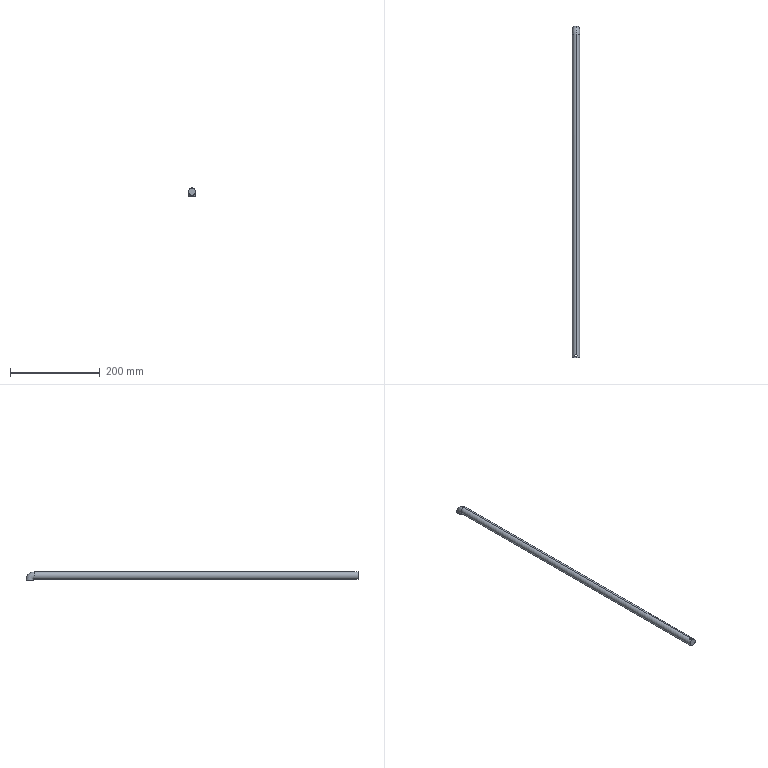Part | SolidWorks | features ICE 2, Sweep 1 | 1 solid | 19 faces | box 16 x 738 x 18 mm | volume 127006 mm3 | cylinder 12 | torus 4 | plane 3 | commonest cylinder face diameters 5 x4 6 x4 16 x4
STEP:
#1=CARTESIAN_POINT('',(-3.,0.,0.05));
#2=VERTEX_POINT('',#1);
#3=CARTESIAN_POINT('',(0.,3.,0.05));
#4=VERTEX_POINT('',#3);
#5=CARTESIAN_POINT('',(0.,0.,0.05));
#6=DIRECTION('',(0.,0.,-1.));
#7=DIRECTION('',(1.,0.,0.));
#8=AXIS2_PLACEMENT_3D('',#5,#6,#7);
#9=CIRCLE('',#8,3.);
#10=EDGE_CURVE('',#2,#4,#9,.T.);
#11=ORIENTED_EDGE('',*,*,#10,.T.);
#12=CARTESIAN_POINT('',(0.,-9.95,13.));
#13=VERTEX_POINT('',#12);
#14=CARTESIAN_POINT('',(0.,-9.95,0.05));
#15=DIRECTION('',(1.,0.,0.));
#16=DIRECTION('',(0.,0.,-1.));
#17=AXIS2_PLACEMENT_3D('',#14,#15,#16);
#18=CIRCLE('',#17,12.95);
#19=EDGE_CURVE('',#4,#13,#18,.T.);
#20=ORIENTED_EDGE('',*,*,#19,.T.);
#21=CARTESIAN_POINT('',(0.,-9.95,7.));
#22=VERTEX_POINT('',#21);
#23=CARTESIAN_POINT('',(0.,-9.95,10.));
#24=DIRECTION('',(0.,1.,0.));
#25=DIRECTION('',(1.,0.,0.));
#26=AXIS2_PLACEMENT_3D('',#23,#24,#25);
#27=CIRCLE('',#26,3.);
#28=EDGE_CURVE('',#22,#13,#27,.T.);
#29=ORIENTED_EDGE('',*,*,#28,.F.);
#30=CARTESIAN_POINT('',(0.,-3.,0.05));
#31=VERTEX_POINT('',#30);
#32=CARTESIAN_POINT('',(0.,-9.95,0.05));
#33=DIRECTION('',(1.,0.,0.));
#34=DIRECTION('',(0.,0.,-1.));
#35=AXIS2_PLACEMENT_3D('',#32,#33,#34);
#36=CIRCLE('',#35,6.95);
#37=EDGE_CURVE('',#31,#22,#36,.T.);
#38=ORIENTED_EDGE('',*,*,#37,.F.);
#39=CARTESIAN_POINT('',(0.,0.,0.05));
#40=DIRECTION('',(0.,0.,-1.));
#41=DIRECTION('',(1.,0.,0.));
#42=AXIS2_PLACEMENT_3D('',#39,#40,#41);
#43=CIRCLE('',#42,3.);
#44=EDGE_CURVE('',#31,#2,#43,.T.);
#45=ORIENTED_EDGE('',*,*,#44,.T.);
#46=EDGE_LOOP('',(#11,#20,#29,#38,#45));
#47=FACE_OUTER_BOUND('',#46,.T.);
#48=CARTESIAN_POINT('',(0.,-9.95,0.05));
#49=DIRECTION('',(1.,0.,0.));
#50=DIRECTION('',(0.,0.,-1.));
#51=AXIS2_PLACEMENT_3D('',#48,#49,#50);
#52=TOROIDAL_SURFACE('',#51,9.95,3.);
#53=ADVANCED_FACE('',(#47),#52,.F.);
#54=CARTESIAN_POINT('',(8.,0.,0.05));
#55=VERTEX_POINT('',#54);
#56=CARTESIAN_POINT('',(0.,8.,0.05));
#57=VERTEX_POINT('',#56);
#58=CARTESIAN_POINT('',(0.,0.,0.05));
#59=DIRECTION('',(0.,0.,1.));
#60=DIRECTION('',(1.,0.,0.));
#61=AXIS2_PLACEMENT_3D('',#58,#59,#60);
#62=CIRCLE('',#61,8.);
#63=EDGE_CURVE('',#55,#57,#62,.T.);
#64=ORIENTED_EDGE('',*,*,#63,.T.);
#65=CARTESIAN_POINT('',(0.,-9.95,18.));
#66=VERTEX_POINT('',#65);
#67=CARTESIAN_POINT('',(0.,-9.95,0.05));
#68=DIRECTION('',(1.,0.,0.));
#69=DIRECTION('',(0.,0.,-1.));
#70=AXIS2_PLACEMENT_3D('',#67,#68,#69);
#71=CIRCLE('',#70,17.95);
#72=EDGE_CURVE('',#57,#66,#71,.T.);
#73=ORIENTED_EDGE('',*,*,#72,.T.);
#74=CARTESIAN_POINT('',(0.,-9.95,2.));
#75=VERTEX_POINT('',#74);
#76=CARTESIAN_POINT('',(0.,-9.95,10.));
#77=DIRECTION('',(0.,-1.,0.));
#78=DIRECTION('',(1.,0.,0.));
#79=AXIS2_PLACEMENT_3D('',#76,#77,#78);
#80=CIRCLE('',#79,8.);
#81=EDGE_CURVE('',#75,#66,#80,.T.);
#82=ORIENTED_EDGE('',*,*,#81,.F.);
#83=CARTESIAN_POINT('',(0.,-8.,0.05));
#84=VERTEX_POINT('',#83);
#85=CARTESIAN_POINT('',(0.,-9.95,0.05));
#86=DIRECTION('',(1.,0.,0.));
#87=DIRECTION('',(0.,0.,-1.));
#88=AXIS2_PLACEMENT_3D('',#85,#86,#87);
#89=CIRCLE('',#88,1.95);
#90=EDGE_CURVE('',#84,#75,#89,.T.);
#91=ORIENTED_EDGE('',*,*,#90,.F.);
#92=CARTESIAN_POINT('',(0.,0.,0.05));
#93=DIRECTION('',(0.,0.,1.));
#94=DIRECTION('',(1.,0.,0.));
#95=AXIS2_PLACEMENT_3D('',#92,#93,#94);
#96=CIRCLE('',#95,8.);
#97=EDGE_CURVE('',#84,#55,#96,.T.);
#98=ORIENTED_EDGE('',*,*,#97,.T.);
#99=EDGE_LOOP('',(#64,#73,#82,#91,#98));
#100=FACE_OUTER_BOUND('',#99,.T.);
#101=CARTESIAN_POINT('',(0.,-9.95,0.05));
#102=DIRECTION('',(1.,0.,0.));
#103=DIRECTION('',(0.,0.,-1.));
#104=AXIS2_PLACEMENT_3D('',#101,#102,#103);
#105=TOROIDAL_SURFACE('',#104,9.95,8.);
#106=ADVANCED_FACE('',(#100),#105,.T.);
#107=CARTESIAN_POINT('',(0.,-727.,2.));
#108=VERTEX_POINT('',#107);
#109=CARTESIAN_POINT('',(-2.5,-724.5,2.401));
#110=VERTEX_POINT('',#109);
#111=CARTESIAN_POINT('',(0.,-727.,2.));
#112=CARTESIAN_POINT('',(-0.1638,-727.,2.));
#113=CARTESIAN_POINT('',(-0.3284,-726.984,2.005));
#114=CARTESIAN_POINT('',(-0.6528,-726.919,2.025));
#115=CARTESIAN_POINT('',(-0.8091,-726.871,2.04));
#116=CARTESIAN_POINT('',(-1.111,-726.746,2.076));
#117=CARTESIAN_POINT('',(-1.257,-726.667,2.098));
#118=CARTESIAN_POINT('',(-1.527,-726.486,2.146));
#119=CARTESIAN_POINT('',(-1.652,-726.383,2.172));
#120=CARTESIAN_POINT('',(-1.883,-726.152,2.224));
#121=CARTESIAN_POINT('',(-1.987,-726.025,2.25));
#122=CARTESIAN_POINT('',(-2.168,-725.756,2.299));
#123=CARTESIAN_POINT('',(-2.245,-725.612,2.321));
#124=CARTESIAN_POINT('',(-2.372,-725.308,2.359));
#125=CARTESIAN_POINT('',(-2.419,-725.152,2.374));
#126=CARTESIAN_POINT('',(-2.483,-724.831,2.395));
#127=CARTESIAN_POINT('',(-2.5,-724.665,2.401));
#128=CARTESIAN_POINT('',(-2.5,-724.5,2.401));
#129=B_SPLINE_CURVE_WITH_KNOTS('',3,(#111,#112,#113,#114,#115,#116,#117,#118,#119,#120,#121,#122,#123,#124,#125,#126,#127,#128),.UNSPECIFIED.,.F.,.F.,(4,2,2,2,2,2,2,2,4),(0.007866,0.008357,0.008849,0.00934,0.009832,0.01032,0.01081,0.01131,0.0118),.UNSPECIFIED.);
#130=EDGE_CURVE('',#108,#110,#129,.T.);
#131=ORIENTED_EDGE('',*,*,#130,.T.);
#132=CARTESIAN_POINT('',(-2.5,-724.5,8.342));
#133=VERTEX_POINT('',#132);
#134=CARTESIAN_POINT('',(-2.5,-724.5,-0.000012));
#135=DIRECTION('',(0.,0.,1.));
#136=VECTOR('',#135,1000.);
#137=LINE('',#134,#136);
#138=EDGE_CURVE('',#110,#133,#137,.T.);
#139=ORIENTED_EDGE('',*,*,#138,.T.);
#140=CARTESIAN_POINT('',(0.,-727.,7.));
#141=VERTEX_POINT('',#140);
#142=CARTESIAN_POINT('',(-2.5,-724.5,8.342));
#143=CARTESIAN_POINT('',(-2.5,-724.674,8.342));
#144=CARTESIAN_POINT('',(-2.481,-724.85,8.312));
#145=CARTESIAN_POINT('',(-2.412,-725.178,8.215));
#146=CARTESIAN_POINT('',(-2.362,-725.335,8.148));
#147=CARTESIAN_POINT('',(-2.238,-725.626,7.999));
#148=CARTESIAN_POINT('',(-2.164,-725.761,7.919));
#149=CARTESIAN_POINT('',(-1.993,-726.017,7.755));
#150=CARTESIAN_POINT('',(-1.895,-726.138,7.67));
#151=CARTESIAN_POINT('',(-1.679,-726.359,7.51));
#152=CARTESIAN_POINT('',(-1.56,-726.46,7.433));
#153=CARTESIAN_POINT('',(-1.299,-726.642,7.292));
#154=CARTESIAN_POINT('',(-1.155,-726.723,7.226));
#155=CARTESIAN_POINT('',(-0.8512,-726.856,7.119));
#156=CARTESIAN_POINT('',(-0.6885,-726.91,7.075));
#157=CARTESIAN_POINT('',(-0.3498,-726.981,7.016));
#158=CARTESIAN_POINT('',(-0.1766,-727.,7.));
#159=CARTESIAN_POINT('',(0.,-727.,7.));
#160=B_SPLINE_CURVE_WITH_KNOTS('',3,(#142,#143,#144,#145,#146,#147,#148,#149,#150,#151,#152,#153,#154,#155,#156,#157,#158,#159),.UNSPECIFIED.,.F.,.F.,(4,2,2,2,2,2,2,2,4),(0.01252,0.01304,0.01356,0.01408,0.0146,0.01512,0.01564,0.01616,0.01668),.UNSPECIFIED.);
#161=EDGE_CURVE('',#133,#141,#160,.T.);
#162=ORIENTED_EDGE('',*,*,#161,.T.);
#163=CARTESIAN_POINT('',(2.5,-724.5,8.342));
#164=VERTEX_POINT('',#163);
#165=CARTESIAN_POINT('',(0.,-727.,7.));
#166=CARTESIAN_POINT('',(0.1768,-727.,7.));
#167=CARTESIAN_POINT('',(0.3491,-726.981,7.015));
#168=CARTESIAN_POINT('',(0.6857,-726.91,7.074));
#169=CARTESIAN_POINT('',(0.8499,-726.857,7.118));
#170=CARTESIAN_POINT('',(1.154,-726.724,7.226));
#171=CARTESIAN_POINT('',(1.298,-726.643,7.291));
#172=CARTESIAN_POINT('',(1.56,-726.46,7.433));
#173=CARTESIAN_POINT('',(1.678,-726.359,7.51));
#174=CARTESIAN_POINT('',(1.895,-726.138,7.67));
#175=CARTESIAN_POINT('',(1.993,-726.017,7.754));
#176=CARTESIAN_POINT('',(2.164,-725.761,7.919));
#177=CARTESIAN_POINT('',(2.238,-725.626,7.999));
#178=CARTESIAN_POINT('',(2.361,-725.336,8.147));
#179=CARTESIAN_POINT('',(2.412,-725.179,8.215));
#180=CARTESIAN_POINT('',(2.481,-724.85,8.312));
#181=CARTESIAN_POINT('',(2.5,-724.674,8.342));
#182=CARTESIAN_POINT('',(2.5,-724.5,8.342));
#183=B_SPLINE_CURVE_WITH_KNOTS('',3,(#165,#166,#167,#168,#169,#170,#171,#172,#173,#174,#175,#176,#177,#178,#179,#180,#181,#182),.UNSPECIFIED.,.F.,.F.,(4,2,2,2,2,2,2,2,4),(0.,0.0005216,0.001043,0.001565,0.002086,0.002608,0.00313,0.003651,0.004173),.UNSPECIFIED.);
#184=EDGE_CURVE('',#141,#164,#183,.T.);
#185=ORIENTED_EDGE('',*,*,#184,.T.);
#186=CARTESIAN_POINT('',(2.5,-724.5,2.401));
#187=VERTEX_POINT('',#186);
#188=CARTESIAN_POINT('',(2.5,-724.5,-0.000012));
#189=DIRECTION('',(0.,0.,1.));
#190=VECTOR('',#189,1000.);
#191=LINE('',#188,#190);
#192=EDGE_CURVE('',#187,#164,#191,.T.);
#193=ORIENTED_EDGE('',*,*,#192,.F.);
#194=CARTESIAN_POINT('',(2.5,-724.5,2.401));
#195=CARTESIAN_POINT('',(2.5,-724.664,2.401));
#196=CARTESIAN_POINT('',(2.483,-724.831,2.395));
#197=CARTESIAN_POINT('',(2.419,-725.152,2.374));
#198=CARTESIAN_POINT('',(2.371,-725.309,2.359));
#199=CARTESIAN_POINT('',(2.245,-725.613,2.321));
#200=CARTESIAN_POINT('',(2.167,-725.757,2.299));
#201=CARTESIAN_POINT('',(1.986,-726.026,2.25));
#202=CARTESIAN_POINT('',(1.882,-726.154,2.224));
#203=CARTESIAN_POINT('',(1.651,-726.384,2.171));
#204=CARTESIAN_POINT('',(1.526,-726.487,2.146));
#205=CARTESIAN_POINT('',(1.256,-726.668,2.098));
#206=CARTESIAN_POINT('',(1.11,-726.746,2.076));
#207=CARTESIAN_POINT('',(0.8087,-726.871,2.04));
#208=CARTESIAN_POINT('',(0.6527,-726.919,2.025));
#209=CARTESIAN_POINT('',(0.3296,-726.984,2.005));
#210=CARTESIAN_POINT('',(0.1638,-727.,2.));
#211=CARTESIAN_POINT('',(0.,-727.,2.));
#212=B_SPLINE_CURVE_WITH_KNOTS('',3,(#194,#195,#196,#197,#198,#199,#200,#201,#202,#203,#204,#205,#206,#207,#208,#209,#210,#211),.UNSPECIFIED.,.F.,.F.,(4,2,2,2,2,2,2,2,4),(0.003934,0.004425,0.004917,0.005408,0.0059,0.006391,0.006883,0.007374,0.007866),.UNSPECIFIED.);
#213=EDGE_CURVE('',#187,#108,#212,.T.);
#214=ORIENTED_EDGE('',*,*,#213,.T.);
#215=EDGE_LOOP('',(#131,#139,#162,#185,#193,#214));
#216=FACE_OUTER_BOUND('',#215,.T.);
#217=CARTESIAN_POINT('',(0.,-724.5,-0.000012));
#218=DIRECTION('',(0.,0.,1.));
#219=DIRECTION('',(1.,0.,0.));
#220=AXIS2_PLACEMENT_3D('',#217,#218,#219);
#221=CYLINDRICAL_SURFACE('',#220,2.5);
#222=ADVANCED_FACE('',(#216),#221,.F.);
#223=CARTESIAN_POINT('',(0.,-727.,13.));
#224=VERTEX_POINT('',#223);
#225=CARTESIAN_POINT('',(-2.5,-724.5,11.658));
#226=VERTEX_POINT('',#225);
#227=CARTESIAN_POINT('',(0.,-727.,13.));
#228=CARTESIAN_POINT('',(-0.1768,-727.,13.));
#229=CARTESIAN_POINT('',(-0.3491,-726.981,12.985));
#230=CARTESIAN_POINT('',(-0.6857,-726.91,12.926));
#231=CARTESIAN_POINT('',(-0.8499,-726.857,12.882));
#232=CARTESIAN_POINT('',(-1.154,-726.724,12.774));
#233=CARTESIAN_POINT('',(-1.298,-726.643,12.709));
#234=CARTESIAN_POINT('',(-1.56,-726.46,12.567));
#235=CARTESIAN_POINT('',(-1.678,-726.359,12.49));
#236=CARTESIAN_POINT('',(-1.895,-726.138,12.33));
#237=CARTESIAN_POINT('',(-1.993,-726.017,12.246));
#238=CARTESIAN_POINT('',(-2.164,-725.761,12.081));
#239=CARTESIAN_POINT('',(-2.238,-725.626,12.001));
#240=CARTESIAN_POINT('',(-2.361,-725.336,11.853));
#241=CARTESIAN_POINT('',(-2.412,-725.179,11.785));
#242=CARTESIAN_POINT('',(-2.481,-724.85,11.688));
#243=CARTESIAN_POINT('',(-2.5,-724.674,11.658));
#244=CARTESIAN_POINT('',(-2.5,-724.5,11.658));
#245=B_SPLINE_CURVE_WITH_KNOTS('',3,(#227,#228,#229,#230,#231,#232,#233,#234,#235,#236,#237,#238,#239,#240,#241,#242,#243,#244),.UNSPECIFIED.,.F.,.F.,(4,2,2,2,2,2,2,2,4),(0.,0.0005216,0.001043,0.001565,0.002086,0.002608,0.00313,0.003651,0.004173),.UNSPECIFIED.);
#246=EDGE_CURVE('',#224,#226,#245,.T.);
#247=ORIENTED_EDGE('',*,*,#246,.T.);
#248=CARTESIAN_POINT('',(-2.5,-724.5,17.599));
#249=VERTEX_POINT('',#248);
#250=CARTESIAN_POINT('',(-2.5,-724.5,-0.000012));
#251=DIRECTION('',(0.,0.,1.));
#252=VECTOR('',#251,1000.);
#253=LINE('',#250,#252);
#254=EDGE_CURVE('',#226,#249,#253,.T.);
#255=ORIENTED_EDGE('',*,*,#254,.T.);
#256=CARTESIAN_POINT('',(0.,-727.,18.));
#257=VERTEX_POINT('',#256);
#258=CARTESIAN_POINT('',(-2.5,-724.5,17.599));
#259=CARTESIAN_POINT('',(-2.5,-724.664,17.599));
#260=CARTESIAN_POINT('',(-2.484,-724.828,17.605));
#261=CARTESIAN_POINT('',(-2.419,-725.153,17.626));
#262=CARTESIAN_POINT('',(-2.371,-725.309,17.641));
#263=CARTESIAN_POINT('',(-2.246,-725.61,17.679));
#264=CARTESIAN_POINT('',(-2.167,-725.757,17.701));
#265=CARTESIAN_POINT('',(-1.986,-726.027,17.75));
#266=CARTESIAN_POINT('',(-1.884,-726.152,17.776));
#267=CARTESIAN_POINT('',(-1.653,-726.383,17.828));
#268=CARTESIAN_POINT('',(-1.526,-726.487,17.854));
#269=CARTESIAN_POINT('',(-1.256,-726.667,17.902));
#270=CARTESIAN_POINT('',(-1.113,-726.745,17.924));
#271=CARTESIAN_POINT('',(-0.8081,-726.872,17.961));
#272=CARTESIAN_POINT('',(-0.6518,-726.919,17.975));
#273=CARTESIAN_POINT('',(-0.3311,-726.983,17.995));
#274=CARTESIAN_POINT('',(-0.1647,-727.,18.));
#275=CARTESIAN_POINT('',(0.,-727.,18.));
#276=B_SPLINE_CURVE_WITH_KNOTS('',3,(#258,#259,#260,#261,#262,#263,#264,#265,#266,#267,#268,#269,#270,#271,#272,#273,#274,#275),.UNSPECIFIED.,.F.,.F.,(4,2,2,2,2,2,2,2,4),(0.007866,0.008357,0.008848,0.00934,0.009831,0.01032,0.01081,0.01131,0.0118),.UNSPECIFIED.);
#277=EDGE_CURVE('',#249,#257,#276,.T.);
#278=ORIENTED_EDGE('',*,*,#277,.T.);
#279=CARTESIAN_POINT('',(2.5,-724.5,17.599));
#280=VERTEX_POINT('',#279);
#281=CARTESIAN_POINT('',(0.,-727.,18.));
#282=CARTESIAN_POINT('',(0.1647,-727.,18.));
#283=CARTESIAN_POINT('',(0.3277,-726.984,17.995));
#284=CARTESIAN_POINT('',(0.6503,-726.92,17.975));
#285=CARTESIAN_POINT('',(0.8096,-726.871,17.96));
#286=CARTESIAN_POINT('',(1.261,-726.683,17.906));
#287=CARTESIAN_POINT('',(1.538,-726.497,17.854));
#288=CARTESIAN_POINT('',(1.882,-726.153,17.776));
#289=CARTESIAN_POINT('',(1.987,-726.026,17.75));
#290=CARTESIAN_POINT('',(2.168,-725.755,17.701));
#291=CARTESIAN_POINT('',(2.245,-725.612,17.679));
#292=CARTESIAN_POINT('',(2.371,-725.311,17.641));
#293=CARTESIAN_POINT('',(2.419,-725.151,17.625));
#294=CARTESIAN_POINT('',(2.484,-724.83,17.605));
#295=CARTESIAN_POINT('',(2.5,-724.666,17.599));
#296=CARTESIAN_POINT('',(2.5,-724.5,17.599));
#297=B_SPLINE_CURVE_WITH_KNOTS('',3,(#281,#282,#283,#284,#285,#286,#287,#288,#289,#290,#291,#292,#293,#294,#295,#296),.UNSPECIFIED.,.F.,.F.,(4,2,2,2,2,2,2,4),(0.0118,0.01229,0.01278,0.01376,0.01425,0.01475,0.01524,0.01573),.UNSPECIFIED.);
#298=EDGE_CURVE('',#257,#280,#297,.T.);
#299=ORIENTED_EDGE('',*,*,#298,.T.);
#300=CARTESIAN_POINT('',(2.5,-724.5,11.658));
#301=VERTEX_POINT('',#300);
#302=CARTESIAN_POINT('',(2.5,-724.5,-0.000012));
#303=DIRECTION('',(0.,0.,1.));
#304=VECTOR('',#303,1000.);
#305=LINE('',#302,#304);
#306=EDGE_CURVE('',#301,#280,#305,.T.);
#307=ORIENTED_EDGE('',*,*,#306,.F.);
#308=CARTESIAN_POINT('',(2.5,-724.5,11.658));
#309=CARTESIAN_POINT('',(2.5,-724.674,11.658));
#310=CARTESIAN_POINT('',(2.481,-724.85,11.688));
#311=CARTESIAN_POINT('',(2.412,-725.178,11.785));
#312=CARTESIAN_POINT('',(2.362,-725.335,11.852));
#313=CARTESIAN_POINT('',(2.238,-725.626,12.001));
#314=CARTESIAN_POINT('',(2.164,-725.761,12.081));
#315=CARTESIAN_POINT('',(1.993,-726.017,12.245));
#316=CARTESIAN_POINT('',(1.895,-726.138,12.33));
#317=CARTESIAN_POINT('',(1.679,-726.359,12.49));
#318=CARTESIAN_POINT('',(1.56,-726.46,12.567));
#319=CARTESIAN_POINT('',(1.299,-726.642,12.708));
#320=CARTESIAN_POINT('',(1.155,-726.723,12.774));
#321=CARTESIAN_POINT('',(0.8512,-726.856,12.881));
#322=CARTESIAN_POINT('',(0.6885,-726.91,12.925));
#323=CARTESIAN_POINT('',(0.3498,-726.981,12.984));
#324=CARTESIAN_POINT('',(0.1766,-727.,13.));
#325=CARTESIAN_POINT('',(0.,-727.,13.));
#326=B_SPLINE_CURVE_WITH_KNOTS('',3,(#308,#309,#310,#311,#312,#313,#314,#315,#316,#317,#318,#319,#320,#321,#322,#323,#324,#325),.UNSPECIFIED.,.F.,.F.,(4,2,2,2,2,2,2,2,4),(0.01252,0.01304,0.01356,0.01408,0.0146,0.01512,0.01564,0.01616,0.01668),.UNSPECIFIED.);
#327=EDGE_CURVE('',#301,#224,#326,.T.);
#328=ORIENTED_EDGE('',*,*,#327,.T.);
#329=EDGE_LOOP('',(#247,#255,#278,#299,#307,#328));
#330=FACE_OUTER_BOUND('',#329,.T.);
#331=CARTESIAN_POINT('',(0.,-724.5,-0.000012));
#332=DIRECTION('',(0.,0.,1.));
#333=DIRECTION('',(1.,0.,0.));
#334=AXIS2_PLACEMENT_3D('',#331,#332,#333);
#335=CYLINDRICAL_SURFACE('',#334,2.5);
#336=ADVANCED_FACE('',(#330),#335,.F.);
#337=CARTESIAN_POINT('',(3.,0.,0.));
#338=VERTEX_POINT('',#337);
#339=CARTESIAN_POINT('',(-3.,0.,0.));
#340=VERTEX_POINT('',#339);
#341=CARTESIAN_POINT('',(0.,0.,0.));
#342=DIRECTION('',(0.,0.,-1.));
#343=DIRECTION('',(1.,0.,0.));
#344=AXIS2_PLACEMENT_3D('',#341,#342,#343);
#345=CIRCLE('',#344,3.);
#346=EDGE_CURVE('',#338,#340,#345,.T.);
#347=ORIENTED_EDGE('',*,*,#346,.T.);
#348=CARTESIAN_POINT('',(-3.,0.,0.));
#349=DIRECTION('',(0.,0.,1.));
#350=VECTOR('',#349,1000.);
#351=LINE('',#348,#350);
#352=EDGE_CURVE('',#340,#2,#351,.T.);
#353=ORIENTED_EDGE('',*,*,#352,.T.);
#354=ORIENTED_EDGE('',*,*,#44,.F.);
#355=CARTESIAN_POINT('',(3.,0.,0.05));
#356=VERTEX_POINT('',#355);
#357=CARTESIAN_POINT('',(0.,0.,0.05));
#358=DIRECTION('',(0.,0.,-1.));
#359=DIRECTION('',(1.,0.,0.));
#360=AXIS2_PLACEMENT_3D('',#357,#358,#359);
#361=CIRCLE('',#360,3.);
#362=EDGE_CURVE('',#356,#31,#361,.T.);
#363=ORIENTED_EDGE('',*,*,#362,.F.);
#364=CARTESIAN_POINT('',(3.,0.,0.));
#365=DIRECTION('',(0.,0.,1.));
#366=VECTOR('',#365,1000.);
#367=LINE('',#364,#366);
#368=EDGE_CURVE('',#338,#356,#367,.T.);
#369=ORIENTED_EDGE('',*,*,#368,.F.);
#370=EDGE_LOOP('',(#347,#353,#354,#363,#369));
#371=FACE_OUTER_BOUND('',#370,.T.);
#372=CARTESIAN_POINT('',(0.,0.,0.));
#373=DIRECTION('',(0.,0.,1.));
#374=DIRECTION('',(1.,0.,0.));
#375=AXIS2_PLACEMENT_3D('',#372,#373,#374);
#376=CYLINDRICAL_SURFACE('',#375,3.);
#377=ADVANCED_FACE('',(#371),#376,.F.);
#378=ORIENTED_EDGE('',*,*,#81,.T.);
#379=CARTESIAN_POINT('',(0.,-722.,18.));
#380=VERTEX_POINT('',#379);
#381=CARTESIAN_POINT('',(0.,-9.95,18.));
#382=DIRECTION('',(0.,-1.,0.));
#383=VECTOR('',#382,1000.);
#384=LINE('',#381,#383);
#385=EDGE_CURVE('',#66,#380,#384,.T.);
#386=ORIENTED_EDGE('',*,*,#385,.T.);
#387=CARTESIAN_POINT('',(2.5,-724.5,17.599));
#388=CARTESIAN_POINT('',(2.5,-724.334,17.599));
#389=CARTESIAN_POINT('',(2.484,-724.17,17.605));
#390=CARTESIAN_POINT('',(2.419,-723.849,17.625));
#391=CARTESIAN_POINT('',(2.371,-723.69,17.641));
#392=CARTESIAN_POINT('',(2.245,-723.388,17.679));
#393=CARTESIAN_POINT('',(2.168,-723.244,17.701));
#394=CARTESIAN_POINT('',(1.986,-722.973,17.75));
#395=CARTESIAN_POINT('',(1.882,-722.846,17.776));
#396=CARTESIAN_POINT('',(1.538,-722.502,17.854));
#397=CARTESIAN_POINT('',(1.26,-722.317,17.906));
#398=CARTESIAN_POINT('',(0.8095,-722.129,17.96));
#399=CARTESIAN_POINT('',(0.6507,-722.081,17.975));
#400=CARTESIAN_POINT('',(0.3273,-722.016,17.995));
#401=CARTESIAN_POINT('',(0.1643,-722.,18.));
#402=CARTESIAN_POINT('',(0.,-722.,18.));
#403=B_SPLINE_CURVE_WITH_KNOTS('',3,(#387,#388,#389,#390,#391,#392,#393,#394,#395,#396,#397,#398,#399,#400,#401,#402),.UNSPECIFIED.,.F.,.F.,(4,2,2,2,2,2,2,4),(0.,0.0004917,0.0009835,0.001475,0.001967,0.00295,0.003442,0.003934),.UNSPECIFIED.);
#404=EDGE_CURVE('',#280,#380,#403,.T.);
#405=ORIENTED_EDGE('',*,*,#404,.F.);
#406=ORIENTED_EDGE('',*,*,#298,.F.);
#407=CARTESIAN_POINT('',(0.,-730.,18.));
#408=VERTEX_POINT('',#407);
#409=CARTESIAN_POINT('',(0.,-9.95,18.));
#410=DIRECTION('',(0.,-1.,0.));
#411=VECTOR('',#410,1000.);
#412=LINE('',#409,#411);
#413=EDGE_CURVE('',#257,#408,#412,.T.);
#414=ORIENTED_EDGE('',*,*,#413,.T.);
#415=CARTESIAN_POINT('',(0.,-730.,2.));
#416=VERTEX_POINT('',#415);
#417=CARTESIAN_POINT('',(0.,-730.,10.));
#418=DIRECTION('',(0.,-1.,0.));
#419=DIRECTION('',(1.,0.,0.));
#420=AXIS2_PLACEMENT_3D('',#417,#418,#419);
#421=CIRCLE('',#420,8.);
#422=EDGE_CURVE('',#416,#408,#421,.T.);
#423=ORIENTED_EDGE('',*,*,#422,.F.);
#424=CARTESIAN_POINT('',(0.,-9.95,2.));
#425=DIRECTION('',(0.,-1.,0.));
#426=VECTOR('',#425,1000.);
#427=LINE('',#424,#426);
#428=EDGE_CURVE('',#108,#416,#427,.T.);
#429=ORIENTED_EDGE('',*,*,#428,.F.);
#430=ORIENTED_EDGE('',*,*,#213,.F.);
#431=CARTESIAN_POINT('',(0.,-722.,2.));
#432=VERTEX_POINT('',#431);
#433=CARTESIAN_POINT('',(0.,-722.,2.));
#434=CARTESIAN_POINT('',(0.1664,-722.,2.));
#435=CARTESIAN_POINT('',(0.3297,-722.016,2.005));
#436=CARTESIAN_POINT('',(0.6508,-722.081,2.025));
#437=CARTESIAN_POINT('',(0.8102,-722.129,2.04));
#438=CARTESIAN_POINT('',(1.113,-722.255,2.076));
#439=CARTESIAN_POINT('',(1.256,-722.332,2.098));
#440=CARTESIAN_POINT('',(1.527,-722.514,2.146));
#441=CARTESIAN_POINT('',(1.654,-722.619,2.172));
#442=CARTESIAN_POINT('',(1.998,-722.963,2.25));
#443=CARTESIAN_POINT('',(2.184,-723.24,2.303));
#444=CARTESIAN_POINT('',(2.371,-723.691,2.359));
#445=CARTESIAN_POINT('',(2.419,-723.849,2.375));
#446=CARTESIAN_POINT('',(2.484,-724.173,2.395));
#447=CARTESIAN_POINT('',(2.5,-724.336,2.401));
#448=CARTESIAN_POINT('',(2.5,-724.5,2.401));
#449=B_SPLINE_CURVE_WITH_KNOTS('',3,(#433,#434,#435,#436,#437,#438,#439,#440,#441,#442,#443,#444,#445,#446,#447,#448),.UNSPECIFIED.,.F.,.F.,(4,2,2,2,2,2,2,4),(0.,0.0004918,0.0009835,0.001475,0.001967,0.002951,0.003442,0.003934),.UNSPECIFIED.);
#450=EDGE_CURVE('',#432,#187,#449,.T.);
#451=ORIENTED_EDGE('',*,*,#450,.F.);
#452=CARTESIAN_POINT('',(0.,-9.95,2.));
#453=DIRECTION('',(0.,-1.,0.));
#454=VECTOR('',#453,1000.);
#455=LINE('',#452,#454);
#456=EDGE_CURVE('',#75,#432,#455,.T.);
#457=ORIENTED_EDGE('',*,*,#456,.F.);
#458=EDGE_LOOP('',(#378,#386,#405,#406,#414,#423,#429,#430,#451,#457));
#459=FACE_OUTER_BOUND('',#458,.T.);
#460=CARTESIAN_POINT('',(0.,-9.95,10.));
#461=DIRECTION('',(0.,-1.,0.));
#462=DIRECTION('',(0.,0.,-1.));
#463=AXIS2_PLACEMENT_3D('',#460,#461,#462);
#464=CYLINDRICAL_SURFACE('',#463,8.);
#465=ADVANCED_FACE('',(#459),#464,.T.);
#466=CARTESIAN_POINT('',(8.,0.,0.));
#467=VERTEX_POINT('',#466);
#468=CARTESIAN_POINT('',(-8.,0.,0.));
#469=VERTEX_POINT('',#468);
#470=CARTESIAN_POINT('',(0.,0.,0.));
#471=DIRECTION('',(0.,0.,1.));
#472=DIRECTION('',(1.,0.,0.));
#473=AXIS2_PLACEMENT_3D('',#470,#471,#472);
#474=CIRCLE('',#473,8.);
#475=EDGE_CURVE('',#467,#469,#474,.T.);
#476=ORIENTED_EDGE('',*,*,#475,.T.);
#477=CARTESIAN_POINT('',(-8.,0.,0.05));
#478=VERTEX_POINT('',#477);
#479=CARTESIAN_POINT('',(-8.,0.,0.));
#480=DIRECTION('',(0.,0.,1.));
#481=VECTOR('',#480,1000.);
#482=LINE('',#479,#481);
#483=EDGE_CURVE('',#469,#478,#482,.T.);
#484=ORIENTED_EDGE('',*,*,#483,.T.);
#485=CARTESIAN_POINT('',(0.,0.,0.05));
#486=DIRECTION('',(0.,0.,1.));
#487=DIRECTION('',(1.,0.,0.));
#488=AXIS2_PLACEMENT_3D('',#485,#486,#487);
#489=CIRCLE('',#488,8.);
#490=EDGE_CURVE('',#57,#478,#489,.T.);
#491=ORIENTED_EDGE('',*,*,#490,.F.);
#492=ORIENTED_EDGE('',*,*,#63,.F.);
#493=CARTESIAN_POINT('',(8.,0.,0.));
#494=DIRECTION('',(0.,0.,1.));
#495=VECTOR('',#494,1000.);
#496=LINE('',#493,#495);
#497=EDGE_CURVE('',#467,#55,#496,.T.);
#498=ORIENTED_EDGE('',*,*,#497,.F.);
#499=EDGE_LOOP('',(#476,#484,#491,#492,#498));
#500=FACE_OUTER_BOUND('',#499,.T.);
#501=CARTESIAN_POINT('',(0.,0.,0.));
#502=DIRECTION('',(0.,0.,1.));
#503=DIRECTION('',(1.,0.,0.));
#504=AXIS2_PLACEMENT_3D('',#501,#502,#503);
#505=CYLINDRICAL_SURFACE('',#504,8.);
#506=ADVANCED_FACE('',(#500),#505,.T.);
#507=ORIENTED_EDGE('',*,*,#28,.T.);
#508=CARTESIAN_POINT('',(0.,-722.,13.));
#509=VERTEX_POINT('',#508);
#510=CARTESIAN_POINT('',(0.,-9.95,13.));
#511=DIRECTION('',(0.,-1.,0.));
#512=VECTOR('',#511,1000.);
#513=LINE('',#510,#512);
#514=EDGE_CURVE('',#13,#509,#513,.T.);
#515=ORIENTED_EDGE('',*,*,#514,.T.);
#516=CARTESIAN_POINT('',(-2.5,-724.5,11.658));
#517=CARTESIAN_POINT('',(-2.5,-724.326,11.658));
#518=CARTESIAN_POINT('',(-2.481,-724.15,11.688));
#519=CARTESIAN_POINT('',(-2.412,-723.821,11.785));
#520=CARTESIAN_POINT('',(-2.362,-723.665,11.853));
#521=CARTESIAN_POINT('',(-2.237,-723.373,12.001));
#522=CARTESIAN_POINT('',(-2.164,-723.238,12.082));
#523=CARTESIAN_POINT('',(-1.992,-722.982,12.246));
#524=CARTESIAN_POINT('',(-1.894,-722.861,12.33));
#525=CARTESIAN_POINT('',(-1.678,-722.64,12.491));
#526=CARTESIAN_POINT('',(-1.559,-722.539,12.567));
#527=CARTESIAN_POINT('',(-1.297,-722.357,12.709));
#528=CARTESIAN_POINT('',(-1.153,-722.275,12.774));
#529=CARTESIAN_POINT('',(-0.8488,-722.143,12.882));
#530=CARTESIAN_POINT('',(-0.685,-722.09,12.926));
#531=CARTESIAN_POINT('',(-0.3474,-722.018,12.985));
#532=CARTESIAN_POINT('',(-0.1754,-722.,13.));
#533=CARTESIAN_POINT('',(0.,-722.,13.));
#534=B_SPLINE_CURVE_WITH_KNOTS('',3,(#516,#517,#518,#519,#520,#521,#522,#523,#524,#525,#526,#527,#528,#529,#530,#531,#532,#533),.UNSPECIFIED.,.F.,.F.,(4,2,2,2,2,2,2,2,4),(0.004173,0.004695,0.005217,0.005738,0.00626,0.006782,0.007304,0.007826,0.008348),.UNSPECIFIED.);
#535=EDGE_CURVE('',#226,#509,#534,.T.);
#536=ORIENTED_EDGE('',*,*,#535,.F.);
#537=ORIENTED_EDGE('',*,*,#246,.F.);
#538=CARTESIAN_POINT('',(0.,-727.,10.));
#539=DIRECTION('',(0.,-1.,0.));
#540=DIRECTION('',(0.,0.,-1.));
#541=AXIS2_PLACEMENT_3D('',#538,#539,#540);
#542=CIRCLE('',#541,3.);
#543=EDGE_CURVE('',#224,#141,#542,.T.);
#544=ORIENTED_EDGE('',*,*,#543,.T.);
#545=ORIENTED_EDGE('',*,*,#161,.F.);
#546=CARTESIAN_POINT('',(0.,-722.,7.));
#547=VERTEX_POINT('',#546);
#548=CARTESIAN_POINT('',(0.,-722.,7.));
#549=CARTESIAN_POINT('',(-0.1751,-722.,7.));
#550=CARTESIAN_POINT('',(-0.3505,-722.019,7.016));
#551=CARTESIAN_POINT('',(-0.6867,-722.09,7.075));
#552=CARTESIAN_POINT('',(-0.8509,-722.143,7.119));
#553=CARTESIAN_POINT('',(-1.155,-722.277,7.227));
#554=CARTESIAN_POINT('',(-1.298,-722.358,7.291));
#555=CARTESIAN_POINT('',(-1.561,-722.54,7.434));
#556=CARTESIAN_POINT('',(-1.679,-722.641,7.51));
#557=CARTESIAN_POINT('',(-1.895,-722.862,7.671));
#558=CARTESIAN_POINT('',(-1.993,-722.983,7.755));
#559=CARTESIAN_POINT('',(-2.164,-723.239,7.919));
#560=CARTESIAN_POINT('',(-2.238,-723.374,8.));
#561=CARTESIAN_POINT('',(-2.361,-723.664,8.147));
#562=CARTESIAN_POINT('',(-2.412,-723.821,8.215));
#563=CARTESIAN_POINT('',(-2.481,-724.15,8.312));
#564=CARTESIAN_POINT('',(-2.5,-724.326,8.342));
#565=CARTESIAN_POINT('',(-2.5,-724.5,8.342));
#566=B_SPLINE_CURVE_WITH_KNOTS('',3,(#548,#549,#550,#551,#552,#553,#554,#555,#556,#557,#558,#559,#560,#561,#562,#563,#564,#565),.UNSPECIFIED.,.F.,.F.,(4,2,2,2,2,2,2,2,4),(0.008348,0.008869,0.00939,0.009911,0.01043,0.01095,0.01147,0.01199,0.01252),.UNSPECIFIED.);
#567=EDGE_CURVE('',#547,#133,#566,.T.);
#568=ORIENTED_EDGE('',*,*,#567,.F.);
#569=CARTESIAN_POINT('',(0.,-9.95,7.));
#570=DIRECTION('',(0.,-1.,0.));
#571=VECTOR('',#570,1000.);
#572=LINE('',#569,#571);
#573=EDGE_CURVE('',#22,#547,#572,.T.);
#574=ORIENTED_EDGE('',*,*,#573,.F.);
#575=EDGE_LOOP('',(#507,#515,#536,#537,#544,#545,#568,#574));
#576=FACE_OUTER_BOUND('',#575,.T.);
#577=CARTESIAN_POINT('',(0.,-9.95,10.));
#578=DIRECTION('',(0.,-1.,0.));
#579=DIRECTION('',(0.,0.,-1.));
#580=AXIS2_PLACEMENT_3D('',#577,#578,#579);
#581=CYLINDRICAL_SURFACE('',#580,3.);
#582=ADVANCED_FACE('',(#576),#581,.F.);
#583=ORIENTED_EDGE('',*,*,#514,.F.);
#584=CARTESIAN_POINT('',(0.,-9.95,10.));
#585=DIRECTION('',(0.,1.,0.));
#586=DIRECTION('',(1.,0.,0.));
#587=AXIS2_PLACEMENT_3D('',#584,#585,#586);
#588=CIRCLE('',#587,3.);
#589=EDGE_CURVE('',#13,#22,#588,.T.);
#590=ORIENTED_EDGE('',*,*,#589,.T.);
#591=ORIENTED_EDGE('',*,*,#573,.T.);
#592=CARTESIAN_POINT('',(2.5,-724.5,8.342));
#593=CARTESIAN_POINT('',(2.5,-724.326,8.342));
#594=CARTESIAN_POINT('',(2.481,-724.15,8.312));
#595=CARTESIAN_POINT('',(2.412,-723.821,8.215));
#596=CARTESIAN_POINT('',(2.362,-723.665,8.147));
#597=CARTESIAN_POINT('',(2.237,-723.373,7.999));
#598=CARTESIAN_POINT('',(2.164,-723.238,7.918));
#599=CARTESIAN_POINT('',(1.992,-722.982,7.754));
#600=CARTESIAN_POINT('',(1.894,-722.861,7.67));
#601=CARTESIAN_POINT('',(1.678,-722.64,7.509));
#602=CARTESIAN_POINT('',(1.559,-722.539,7.433));
#603=CARTESIAN_POINT('',(1.297,-722.357,7.291));
#604=CARTESIAN_POINT('',(1.153,-722.275,7.226));
#605=CARTESIAN_POINT('',(0.8488,-722.143,7.118));
#606=CARTESIAN_POINT('',(0.685,-722.09,7.074));
#607=CARTESIAN_POINT('',(0.3474,-722.018,7.015));
#608=CARTESIAN_POINT('',(0.1754,-722.,7.));
#609=CARTESIAN_POINT('',(0.,-722.,7.));
#610=B_SPLINE_CURVE_WITH_KNOTS('',3,(#592,#593,#594,#595,#596,#597,#598,#599,#600,#601,#602,#603,#604,#605,#606,#607,#608,#609),.UNSPECIFIED.,.F.,.F.,(4,2,2,2,2,2,2,2,4),(0.004173,0.004695,0.005217,0.005738,0.00626,0.006782,0.007304,0.007826,0.008348),.UNSPECIFIED.);
#611=EDGE_CURVE('',#164,#547,#610,.T.);
#612=ORIENTED_EDGE('',*,*,#611,.F.);
#613=ORIENTED_EDGE('',*,*,#184,.F.);
#614=CARTESIAN_POINT('',(0.,-727.,10.));
#615=DIRECTION('',(0.,-1.,0.));
#616=DIRECTION('',(0.,0.,-1.));
#617=AXIS2_PLACEMENT_3D('',#614,#615,#616);
#618=CIRCLE('',#617,3.);
#619=EDGE_CURVE('',#141,#224,#618,.T.);
#620=ORIENTED_EDGE('',*,*,#619,.T.);
#621=ORIENTED_EDGE('',*,*,#327,.F.);
#622=CARTESIAN_POINT('',(0.,-722.,13.));
#623=CARTESIAN_POINT('',(0.1751,-722.,13.));
#624=CARTESIAN_POINT('',(0.3505,-722.019,12.984));
#625=CARTESIAN_POINT('',(0.6867,-722.09,12.925));
#626=CARTESIAN_POINT('',(0.8509,-722.143,12.881));
#627=CARTESIAN_POINT('',(1.155,-722.277,12.773));
#628=CARTESIAN_POINT('',(1.298,-722.358,12.709));
#629=CARTESIAN_POINT('',(1.561,-722.54,12.566));
#630=CARTESIAN_POINT('',(1.679,-722.641,12.49));
#631=CARTESIAN_POINT('',(1.895,-722.862,12.329));
#632=CARTESIAN_POINT('',(1.993,-722.983,12.245));
#633=CARTESIAN_POINT('',(2.164,-723.239,12.081));
#634=CARTESIAN_POINT('',(2.238,-723.374,12.));
#635=CARTESIAN_POINT('',(2.361,-723.664,11.853));
#636=CARTESIAN_POINT('',(2.412,-723.821,11.785));
#637=CARTESIAN_POINT('',(2.481,-724.15,11.688));
#638=CARTESIAN_POINT('',(2.5,-724.326,11.658));
#639=CARTESIAN_POINT('',(2.5,-724.5,11.658));
#640=B_SPLINE_CURVE_WITH_KNOTS('',3,(#622,#623,#624,#625,#626,#627,#628,#629,#630,#631,#632,#633,#634,#635,#636,#637,#638,#639),.UNSPECIFIED.,.F.,.F.,(4,2,2,2,2,2,2,2,4),(0.008348,0.008869,0.00939,0.009911,0.01043,0.01095,0.01147,0.01199,0.01252),.UNSPECIFIED.);
#641=EDGE_CURVE('',#509,#301,#640,.T.);
#642=ORIENTED_EDGE('',*,*,#641,.F.);
#643=EDGE_LOOP('',(#583,#590,#591,#612,#613,#620,#621,#642));
#644=FACE_OUTER_BOUND('',#643,.T.);
#645=CARTESIAN_POINT('',(0.,-9.95,10.));
#646=DIRECTION('',(0.,-1.,0.));
#647=DIRECTION('',(0.,0.,-1.));
#648=AXIS2_PLACEMENT_3D('',#645,#646,#647);
#649=CYLINDRICAL_SURFACE('',#648,3.);
#650=ADVANCED_FACE('',(#644),#649,.F.);
#651=ORIENTED_EDGE('',*,*,#19,.F.);
#652=CARTESIAN_POINT('',(0.,0.,0.05));
#653=DIRECTION('',(0.,0.,-1.));
#654=DIRECTION('',(1.,0.,0.));
#655=AXIS2_PLACEMENT_3D('',#652,#653,#654);
#656=CIRCLE('',#655,3.);
#657=EDGE_CURVE('',#4,#356,#656,.T.);
#658=ORIENTED_EDGE('',*,*,#657,.T.);
#659=ORIENTED_EDGE('',*,*,#362,.T.);
#660=ORIENTED_EDGE('',*,*,#37,.T.);
#661=ORIENTED_EDGE('',*,*,#589,.F.);
#662=EDGE_LOOP('',(#651,#658,#659,#660,#661));
#663=FACE_OUTER_BOUND('',#662,.T.);
#664=CARTESIAN_POINT('',(0.,-9.95,0.05));
#665=DIRECTION('',(1.,0.,0.));
#666=DIRECTION('',(0.,0.,-1.));
#667=AXIS2_PLACEMENT_3D('',#664,#665,#666);
#668=TOROIDAL_SURFACE('',#667,9.95,3.);
#669=ADVANCED_FACE('',(#663),#668,.F.);
#670=ORIENTED_EDGE('',*,*,#352,.F.);
#671=CARTESIAN_POINT('',(0.,0.,0.));
#672=DIRECTION('',(0.,0.,-1.));
#673=DIRECTION('',(1.,0.,0.));
#674=AXIS2_PLACEMENT_3D('',#671,#672,#673);
#675=CIRCLE('',#674,3.);
#676=EDGE_CURVE('',#340,#338,#675,.T.);
#677=ORIENTED_EDGE('',*,*,#676,.T.);
#678=ORIENTED_EDGE('',*,*,#368,.T.);
#679=ORIENTED_EDGE('',*,*,#657,.F.);
#680=ORIENTED_EDGE('',*,*,#10,.F.);
#681=EDGE_LOOP('',(#670,#677,#678,#679,#680));
#682=FACE_OUTER_BOUND('',#681,.T.);
#683=CARTESIAN_POINT('',(0.,0.,0.));
#684=DIRECTION('',(0.,0.,1.));
#685=DIRECTION('',(1.,0.,0.));
#686=AXIS2_PLACEMENT_3D('',#683,#684,#685);
#687=CYLINDRICAL_SURFACE('',#686,3.);
#688=ADVANCED_FACE('',(#682),#687,.F.);
#689=ORIENTED_EDGE('',*,*,#422,.T.);
#690=CARTESIAN_POINT('',(0.,-730.,10.));
#691=DIRECTION('',(0.,-1.,0.));
#692=DIRECTION('',(1.,0.,0.));
#693=AXIS2_PLACEMENT_3D('',#690,#691,#692);
#694=CIRCLE('',#693,8.);
#695=EDGE_CURVE('',#408,#416,#694,.T.);
#696=ORIENTED_EDGE('',*,*,#695,.T.);
#697=EDGE_LOOP('',(#689,#696));
#698=FACE_OUTER_BOUND('',#697,.T.);
#699=CARTESIAN_POINT('',(0.,-730.,10.));
#700=DIRECTION('',(0.,-1.,0.));
#701=DIRECTION('',(1.,0.,0.));
#702=AXIS2_PLACEMENT_3D('',#699,#700,#701);
#703=PLANE('',#702);
#704=ADVANCED_FACE('',(#698),#703,.T.);
#705=ORIENTED_EDGE('',*,*,#346,.F.);
#706=ORIENTED_EDGE('',*,*,#676,.F.);
#707=EDGE_LOOP('',(#705,#706));
#708=FACE_BOUND('',#707,.T.);
#709=ORIENTED_EDGE('',*,*,#475,.F.);
#710=CARTESIAN_POINT('',(0.,0.,0.));
#711=DIRECTION('',(0.,0.,1.));
#712=DIRECTION('',(1.,0.,0.));
#713=AXIS2_PLACEMENT_3D('',#710,#711,#712);
#714=CIRCLE('',#713,8.);
#715=EDGE_CURVE('',#469,#467,#714,.T.);
#716=ORIENTED_EDGE('',*,*,#715,.F.);
#717=EDGE_LOOP('',(#709,#716));
#718=FACE_OUTER_BOUND('',#717,.T.);
#719=CARTESIAN_POINT('',(0.,0.,0.));
#720=DIRECTION('',(0.,0.,1.));
#721=DIRECTION('',(1.,0.,0.));
#722=AXIS2_PLACEMENT_3D('',#719,#720,#721);
#723=PLANE('',#722);
#724=ADVANCED_FACE('',(#708,#718),#723,.F.);
#725=ORIENTED_EDGE('',*,*,#385,.F.);
#726=CARTESIAN_POINT('',(0.,-9.95,10.));
#727=DIRECTION('',(0.,-1.,0.));
#728=DIRECTION('',(1.,0.,0.));
#729=AXIS2_PLACEMENT_3D('',#726,#727,#728);
#730=CIRCLE('',#729,8.);
#731=EDGE_CURVE('',#66,#75,#730,.T.);
#732=ORIENTED_EDGE('',*,*,#731,.T.);
#733=ORIENTED_EDGE('',*,*,#456,.T.);
#734=CARTESIAN_POINT('',(-2.5,-724.5,2.401));
#735=CARTESIAN_POINT('',(-2.5,-724.335,2.401));
#736=CARTESIAN_POINT('',(-2.484,-724.172,2.395));
#737=CARTESIAN_POINT('',(-2.42,-723.85,2.375));
#738=CARTESIAN_POINT('',(-2.371,-723.691,2.359));
#739=CARTESIAN_POINT('',(-2.183,-723.239,2.303));
#740=CARTESIAN_POINT('',(-1.997,-722.962,2.25));
#741=CARTESIAN_POINT('',(-1.654,-722.618,2.172));
#742=CARTESIAN_POINT('',(-1.526,-722.513,2.146));
#743=CARTESIAN_POINT('',(-1.256,-722.332,2.098));
#744=CARTESIAN_POINT('',(-1.113,-722.255,2.076));
#745=CARTESIAN_POINT('',(-0.8108,-722.129,2.04));
#746=CARTESIAN_POINT('',(-0.6512,-722.081,2.025));
#747=CARTESIAN_POINT('',(-0.3297,-722.016,2.005));
#748=CARTESIAN_POINT('',(-0.1663,-722.,2.));
#749=CARTESIAN_POINT('',(0.,-722.,2.));
#750=B_SPLINE_CURVE_WITH_KNOTS('',3,(#734,#735,#736,#737,#738,#739,#740,#741,#742,#743,#744,#745,#746,#747,#748,#749),.UNSPECIFIED.,.F.,.F.,(4,2,2,2,2,2,2,4),(0.0118,0.01229,0.01278,0.01376,0.01425,0.01475,0.01524,0.01573),.UNSPECIFIED.);
#751=EDGE_CURVE('',#110,#432,#750,.T.);
#752=ORIENTED_EDGE('',*,*,#751,.F.);
#753=ORIENTED_EDGE('',*,*,#130,.F.);
#754=ORIENTED_EDGE('',*,*,#428,.T.);
#755=ORIENTED_EDGE('',*,*,#695,.F.);
#756=ORIENTED_EDGE('',*,*,#413,.F.);
#757=ORIENTED_EDGE('',*,*,#277,.F.);
#758=CARTESIAN_POINT('',(0.,-722.,18.));
#759=CARTESIAN_POINT('',(-0.1642,-722.,18.));
#760=CARTESIAN_POINT('',(-0.331,-722.017,17.995));
#761=CARTESIAN_POINT('',(-0.6524,-722.081,17.975));
#762=CARTESIAN_POINT('',(-0.8088,-722.129,17.96));
#763=CARTESIAN_POINT('',(-1.113,-722.255,17.924));
#764=CARTESIAN_POINT('',(-1.257,-722.333,17.902));
#765=CARTESIAN_POINT('',(-1.527,-722.514,17.854));
#766=CARTESIAN_POINT('',(-1.654,-722.618,17.828));
#767=CARTESIAN_POINT('',(-1.884,-722.849,17.776));
#768=CARTESIAN_POINT('',(-1.987,-722.974,17.75));
#769=CARTESIAN_POINT('',(-2.168,-723.244,17.701));
#770=CARTESIAN_POINT('',(-2.246,-723.39,17.678));
#771=CARTESIAN_POINT('',(-2.371,-723.691,17.641));
#772=CARTESIAN_POINT('',(-2.419,-723.847,17.626));
#773=CARTESIAN_POINT('',(-2.484,-724.17,17.605));
#774=CARTESIAN_POINT('',(-2.5,-724.336,17.599));
#775=CARTESIAN_POINT('',(-2.5,-724.5,17.599));
#776=B_SPLINE_CURVE_WITH_KNOTS('',3,(#758,#759,#760,#761,#762,#763,#764,#765,#766,#767,#768,#769,#770,#771,#772,#773,#774,#775),.UNSPECIFIED.,.F.,.F.,(4,2,2,2,2,2,2,2,4),(0.003934,0.004425,0.004917,0.005408,0.0059,0.006391,0.006883,0.007374,0.007866),.UNSPECIFIED.);
#777=EDGE_CURVE('',#380,#249,#776,.T.);
#778=ORIENTED_EDGE('',*,*,#777,.F.);
#779=EDGE_LOOP('',(#725,#732,#733,#752,#753,#754,#755,#756,#757,#778));
#780=FACE_OUTER_BOUND('',#779,.T.);
#781=CARTESIAN_POINT('',(0.,-9.95,10.));
#782=DIRECTION('',(0.,-1.,0.));
#783=DIRECTION('',(0.,0.,-1.));
#784=AXIS2_PLACEMENT_3D('',#781,#782,#783);
#785=CYLINDRICAL_SURFACE('',#784,8.);
#786=ADVANCED_FACE('',(#780),#785,.T.);
#787=ORIENTED_EDGE('',*,*,#72,.F.);
#788=ORIENTED_EDGE('',*,*,#490,.T.);
#789=CARTESIAN_POINT('',(0.,0.,0.05));
#790=DIRECTION('',(0.,0.,1.));
#791=DIRECTION('',(1.,0.,0.));
#792=AXIS2_PLACEMENT_3D('',#789,#790,#791);
#793=CIRCLE('',#792,8.);
#794=EDGE_CURVE('',#478,#84,#793,.T.);
#795=ORIENTED_EDGE('',*,*,#794,.T.);
#796=ORIENTED_EDGE('',*,*,#90,.T.);
#797=ORIENTED_EDGE('',*,*,#731,.F.);
#798=EDGE_LOOP('',(#787,#788,#795,#796,#797));
#799=FACE_OUTER_BOUND('',#798,.T.);
#800=CARTESIAN_POINT('',(0.,-9.95,0.05));
#801=DIRECTION('',(1.,0.,0.));
#802=DIRECTION('',(0.,0.,-1.));
#803=AXIS2_PLACEMENT_3D('',#800,#801,#802);
#804=TOROIDAL_SURFACE('',#803,9.95,8.);
#805=ADVANCED_FACE('',(#799),#804,.T.);
#806=ORIENTED_EDGE('',*,*,#483,.F.);
#807=ORIENTED_EDGE('',*,*,#715,.T.);
#808=ORIENTED_EDGE('',*,*,#497,.T.);
#809=ORIENTED_EDGE('',*,*,#97,.F.);
#810=ORIENTED_EDGE('',*,*,#794,.F.);
#811=EDGE_LOOP('',(#806,#807,#808,#809,#810));
#812=FACE_OUTER_BOUND('',#811,.T.);
#813=CARTESIAN_POINT('',(0.,0.,0.));
#814=DIRECTION('',(0.,0.,1.));
#815=DIRECTION('',(1.,0.,0.));
#816=AXIS2_PLACEMENT_3D('',#813,#814,#815);
#817=CYLINDRICAL_SURFACE('',#816,8.);
#818=ADVANCED_FACE('',(#812),#817,.T.);
#819=ORIENTED_EDGE('',*,*,#619,.F.);
#820=ORIENTED_EDGE('',*,*,#543,.F.);
#821=EDGE_LOOP('',(#819,#820));
#822=FACE_OUTER_BOUND('',#821,.T.);
#823=CARTESIAN_POINT('',(0.,-727.,10.));
#824=DIRECTION('',(0.,-1.,0.));
#825=DIRECTION('',(0.,0.,-1.));
#826=AXIS2_PLACEMENT_3D('',#823,#824,#825);
#827=PLANE('',#826);
#828=ADVANCED_FACE('',(#822),#827,.F.);
#829=ORIENTED_EDGE('',*,*,#254,.F.);
#830=ORIENTED_EDGE('',*,*,#535,.T.);
#831=ORIENTED_EDGE('',*,*,#641,.T.);
#832=ORIENTED_EDGE('',*,*,#306,.T.);
#833=ORIENTED_EDGE('',*,*,#404,.T.);
#834=ORIENTED_EDGE('',*,*,#777,.T.);
#835=EDGE_LOOP('',(#829,#830,#831,#832,#833,#834));
#836=FACE_OUTER_BOUND('',#835,.T.);
#837=CARTESIAN_POINT('',(0.,-724.5,-0.000012));
#838=DIRECTION('',(0.,0.,1.));
#839=DIRECTION('',(1.,0.,0.));
#840=AXIS2_PLACEMENT_3D('',#837,#838,#839);
#841=CYLINDRICAL_SURFACE('',#840,2.5);
#842=ADVANCED_FACE('',(#836),#841,.F.);
#843=ORIENTED_EDGE('',*,*,#138,.F.);
#844=ORIENTED_EDGE('',*,*,#751,.T.);
#845=ORIENTED_EDGE('',*,*,#450,.T.);
#846=ORIENTED_EDGE('',*,*,#192,.T.);
#847=ORIENTED_EDGE('',*,*,#611,.T.);
#848=ORIENTED_EDGE('',*,*,#567,.T.);
#849=EDGE_LOOP('',(#843,#844,#845,#846,#847,#848));
#850=FACE_OUTER_BOUND('',#849,.T.);
#851=CARTESIAN_POINT('',(0.,-724.5,-0.000012));
#852=DIRECTION('',(0.,0.,1.));
#853=DIRECTION('',(1.,0.,0.));
#854=AXIS2_PLACEMENT_3D('',#851,#852,#853);
#855=CYLINDRICAL_SURFACE('',#854,2.5);
#856=ADVANCED_FACE('',(#850),#855,.F.);
#857=CLOSED_SHELL('',(#53,#106,#222,#336,#377,#465,#506,#582,#650,#669,#688,#704,#724,#786,#805,#818,#828,#842,#856));
#858=MANIFOLD_SOLID_BREP('',#857);
#859=CARTESIAN_POINT('',(0.,0.,0.));
#860=DIRECTION('',(0.,0.,1.));
#861=DIRECTION('',(1.,0.,0.));
#862=AXIS2_PLACEMENT_3D('',#859,#860,#861);
#863=(LENGTH_UNIT()NAMED_UNIT(*)SI_UNIT(.MILLI.,.METRE.));
#864=UNCERTAINTY_MEASURE_WITH_UNIT(LENGTH_MEASURE(0.00001),#863,'','');
#865=(NAMED_UNIT(*)PLANE_ANGLE_UNIT()SI_UNIT($,.RADIAN.));
#866=(NAMED_UNIT(*)SI_UNIT($,.STERADIAN.)SOLID_ANGLE_UNIT());
#867=(GEOMETRIC_REPRESENTATION_CONTEXT(3)GLOBAL_UNCERTAINTY_ASSIGNED_CONTEXT((#864))GLOBAL_UNIT_ASSIGNED_CONTEXT((#863,#865,#866))REPRESENTATION_CONTEXT('',''));
#868=ADVANCED_BREP_SHAPE_REPRESENTATION('',(#858,#862),#867);